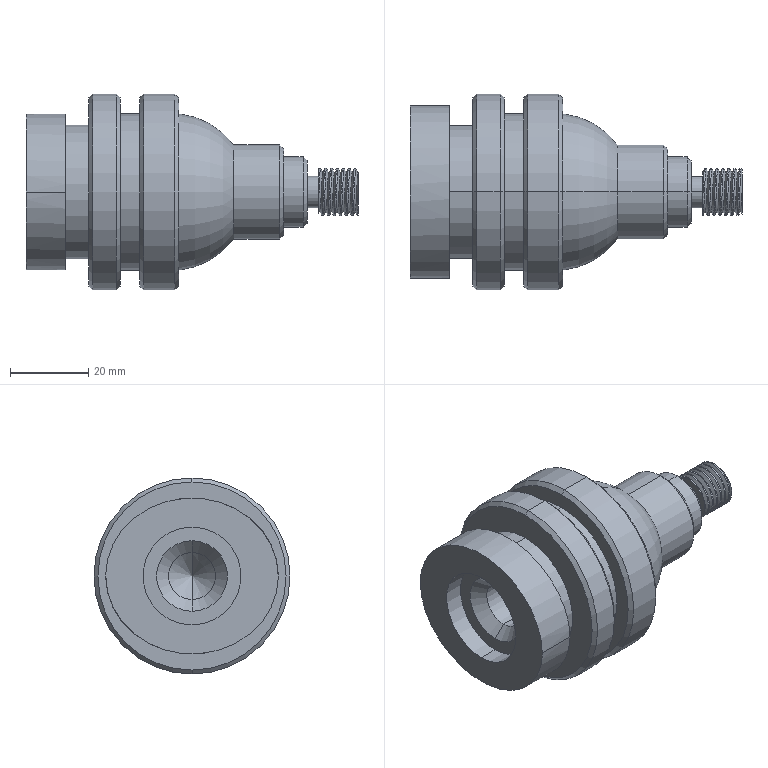Part | SolidWorks | features Chamfer 1, Helix 1, ICE 1, RevCut 1, Revolution 1, SweepCut 1 | 1 solid | 66 faces | box 84.7 x 50 x 50 mm | volume 76525 mm3 | cylinder 33 | cone 16 | plane 11 | spline 4 | torus 2 | commonest cylinder face diameters 12 x17 50 x4 8 x2 18 x2 24 x2 25 x2